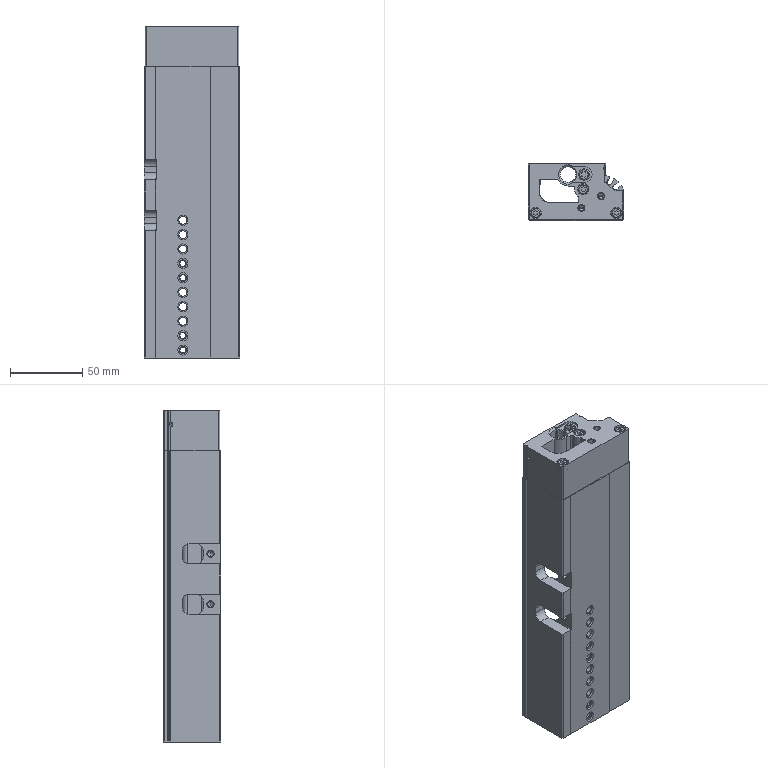Part | SolidWorks | features RefAxis 57, RevCut 21, 3DProfileFeature 19, ICE 16, Revolution 4, Extrusion 1 | 1 solid | 377 faces | box 66 x 39.6 x 230 mm | volume 297307 mm3 | cylinder 172 | plane 148 | cone 57 | commonest cylinder face diameters 0.4 x33 7 x27 4.134 x21 5.5 x12 9 x12 8 x10